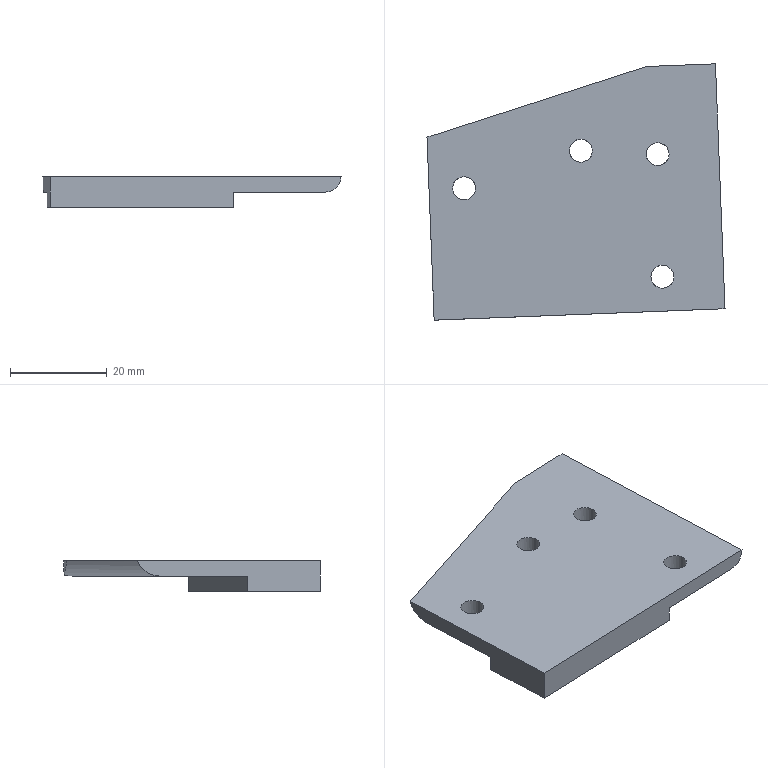Part | NX | features MG0301 nose pivot 24(right) 2 | 1 solid | 14 faces | box 61.764 x 53.123 x 6.35 mm | volume 10727 mm3 | plane 8 | cylinder 6 | commonest cylinder face diameters 4.763 x4 6.35 x1 9.525 x1
STEP:
#1=CARTESIAN_POINT('',(-3.173,-0.1243,6.35));
#2=VERTEX_POINT('',#1);
#3=CARTESIAN_POINT('',(-5.334,-0.209,3.34));
#4=VERTEX_POINT('',#3);
#5=CARTESIAN_POINT('',(-6.345,-0.2486,6.35));
#6=DIRECTION('',(0.03915,-0.9992,0.));
#7=DIRECTION('',(-0.9992,-0.03915,0.));
#8=AXIS2_PLACEMENT_3D('',#5,#6,#7);
#9=CIRCLE('',#8,3.175);
#10=EDGE_CURVE('',#2,#4,#9,.F.);
#11=ORIENTED_EDGE('',*,*,#10,.T.);
#12=CARTESIAN_POINT('',(-17.397,-0.6816,6.35));
#13=VERTEX_POINT('',#12);
#14=CARTESIAN_POINT('',(-0.7099,-0.02781,7.938));
#15=DIRECTION('',(0.03915,-0.9992,0.));
#16=DIRECTION('',(0.9992,0.03915,0.));
#17=AXIS2_PLACEMENT_3D('',#14,#15,#16);
#18=ELLIPSE('',#17,17.713,4.763);
#19=EDGE_CURVE('',#4,#13,#18,.F.);
#20=ORIENTED_EDGE('',*,*,#19,.T.);
#21=CARTESIAN_POINT('',(0.,0.,6.35));
#22=DIRECTION('',(-0.9992,-0.03915,0.));
#23=VECTOR('',#22,1000.);
#24=LINE('',#21,#23);
#25=EDGE_CURVE('',#2,#13,#24,.T.);
#26=ORIENTED_EDGE('',*,*,#25,.F.);
#27=EDGE_LOOP('',(#11,#20,#26));
#28=FACE_BOUND('',#27,.T.);
#29=CARTESIAN_POINT('',(0.,0.,6.35));
#30=DIRECTION('',(-0.03915,0.9992,0.));
#31=DIRECTION('',(-0.9992,-0.03915,0.));
#32=AXIS2_PLACEMENT_3D('',#29,#30,#31);
#33=PLANE('',#32);
#34=ADVANCED_FACE('',(#28),#33,.T.);
#35=CARTESIAN_POINT('',(-23.392,-51.755,0.));
#36=VERTEX_POINT('',#35);
#37=CARTESIAN_POINT('',(-23.392,-51.755,3.175));
#38=VERTEX_POINT('',#37);
#39=CARTESIAN_POINT('',(-23.392,-51.755,6.35));
#40=DIRECTION('',(0.,0.,1.));
#41=VECTOR('',#40,1000.);
#42=LINE('',#39,#41);
#43=EDGE_CURVE('',#36,#38,#42,.T.);
#44=ORIENTED_EDGE('',*,*,#43,.T.);
#45=CARTESIAN_POINT('',(-4.357,-51.01,3.175));
#46=VERTEX_POINT('',#45);
#47=CARTESIAN_POINT('',(-61.463,-53.247,3.175));
#48=DIRECTION('',(0.9992,0.03915,0.));
#49=VECTOR('',#48,1000.);
#50=LINE('',#47,#49);
#51=EDGE_CURVE('',#38,#46,#50,.T.);
#52=ORIENTED_EDGE('',*,*,#51,.T.);
#53=CARTESIAN_POINT('',(-1.184,-50.885,6.35));
#54=VERTEX_POINT('',#53);
#55=CARTESIAN_POINT('',(-4.357,-51.01,6.35));
#56=DIRECTION('',(-0.03915,0.9992,0.));
#57=DIRECTION('',(0.9992,0.03915,0.));
#58=AXIS2_PLACEMENT_3D('',#55,#56,#57);
#59=CIRCLE('',#58,3.175);
#60=EDGE_CURVE('',#46,#54,#59,.F.);
#61=ORIENTED_EDGE('',*,*,#60,.T.);
#62=CARTESIAN_POINT('',(-61.463,-53.247,6.35));
#63=VERTEX_POINT('',#62);
#64=CARTESIAN_POINT('',(-61.463,-53.247,6.35));
#65=DIRECTION('',(0.9992,0.03915,0.));
#66=VECTOR('',#65,1000.);
#67=LINE('',#64,#66);
#68=EDGE_CURVE('',#63,#54,#67,.T.);
#69=ORIENTED_EDGE('',*,*,#68,.F.);
#70=CARTESIAN_POINT('',(-61.463,-53.247,0.));
#71=VERTEX_POINT('',#70);
#72=CARTESIAN_POINT('',(-61.463,-53.247,6.35));
#73=DIRECTION('',(0.,0.,-1.));
#74=VECTOR('',#73,1000.);
#75=LINE('',#72,#74);
#76=EDGE_CURVE('',#63,#71,#75,.T.);
#77=ORIENTED_EDGE('',*,*,#76,.T.);
#78=CARTESIAN_POINT('',(-61.463,-53.247,0.));
#79=DIRECTION('',(0.9992,0.03915,0.));
#80=VECTOR('',#79,1000.);
#81=LINE('',#78,#80);
#82=EDGE_CURVE('',#71,#36,#81,.T.);
#83=ORIENTED_EDGE('',*,*,#82,.T.);
#84=EDGE_LOOP('',(#44,#52,#61,#69,#77,#83));
#85=FACE_BOUND('',#84,.T.);
#86=CARTESIAN_POINT('',(-61.463,-53.247,6.35));
#87=DIRECTION('',(0.03915,-0.9992,0.));
#88=DIRECTION('',(0.9992,0.03915,0.));
#89=AXIS2_PLACEMENT_3D('',#86,#87,#88);
#90=PLANE('',#89);
#91=ADVANCED_FACE('',(#85),#90,.T.);
#92=CARTESIAN_POINT('',(-15.149,-16.459,3.175));
#93=VERTEX_POINT('',#92);
#94=CARTESIAN_POINT('',(-15.149,-18.84,3.175));
#95=DIRECTION('',(0.,0.,-1.));
#96=DIRECTION('',(0.,1.,0.));
#97=AXIS2_PLACEMENT_3D('',#94,#95,#96);
#98=CIRCLE('',#97,2.381);
#99=EDGE_CURVE('',#93,#93,#98,.T.);
#100=ORIENTED_EDGE('',*,*,#99,.F.);
#101=EDGE_LOOP('',(#100));
#102=FACE_BOUND('',#101,.T.);
#103=CARTESIAN_POINT('',(-31.064,-15.754,3.175));
#104=VERTEX_POINT('',#103);
#105=CARTESIAN_POINT('',(-31.064,-18.135,3.175));
#106=DIRECTION('',(0.,0.,-1.));
#107=DIRECTION('',(0.,1.,0.));
#108=AXIS2_PLACEMENT_3D('',#105,#106,#107);
#109=CIRCLE('',#108,2.381);
#110=EDGE_CURVE('',#104,#104,#109,.T.);
#111=ORIENTED_EDGE('',*,*,#110,.F.);
#112=EDGE_LOOP('',(#111));
#113=FACE_BOUND('',#112,.T.);
#114=CARTESIAN_POINT('',(-55.242,-23.536,3.175));
#115=VERTEX_POINT('',#114);
#116=CARTESIAN_POINT('',(-55.242,-25.917,3.175));
#117=DIRECTION('',(0.,0.,-1.));
#118=DIRECTION('',(0.,1.,0.));
#119=AXIS2_PLACEMENT_3D('',#116,#117,#118);
#120=CIRCLE('',#119,2.381);
#121=EDGE_CURVE('',#115,#115,#120,.T.);
#122=ORIENTED_EDGE('',*,*,#121,.F.);
#123=EDGE_LOOP('',(#122));
#124=FACE_BOUND('',#123,.T.);
#125=CARTESIAN_POINT('',(-14.154,-41.859,3.175));
#126=VERTEX_POINT('',#125);
#127=CARTESIAN_POINT('',(-14.154,-44.24,3.175));
#128=DIRECTION('',(0.,0.,-1.));
#129=DIRECTION('',(0.,1.,0.));
#130=AXIS2_PLACEMENT_3D('',#127,#128,#129);
#131=CIRCLE('',#130,2.381);
#132=EDGE_CURVE('',#126,#126,#131,.T.);
#133=ORIENTED_EDGE('',*,*,#132,.F.);
#134=EDGE_LOOP('',(#133));
#135=FACE_BOUND('',#134,.T.);
#136=CARTESIAN_POINT('',(-62.055,-38.116,3.175));
#137=VERTEX_POINT('',#136);
#138=CARTESIAN_POINT('',(-24.401,-25.997,3.175));
#139=VERTEX_POINT('',#138);
#140=CARTESIAN_POINT('',(-468.479,-168.921,3.175));
#141=DIRECTION('',(0.9519,0.3064,0.));
#142=VECTOR('',#141,1000.);
#143=LINE('',#140,#142);
#144=EDGE_CURVE('',#137,#139,#143,.T.);
#145=ORIENTED_EDGE('',*,*,#144,.F.);
#146=CARTESIAN_POINT('',(-62.765,-20.,3.175));
#147=VERTEX_POINT('',#146);
#148=CARTESIAN_POINT('',(-62.959,-15.059,3.175));
#149=DIRECTION('',(0.03915,-0.9992,0.));
#150=VECTOR('',#149,1000.);
#151=LINE('',#148,#150);
#152=EDGE_CURVE('',#147,#137,#151,.T.);
#153=ORIENTED_EDGE('',*,*,#152,.F.);
#154=CARTESIAN_POINT('',(-6.284,-1.822,3.175));
#155=VERTEX_POINT('',#154);
#156=CARTESIAN_POINT('',(-473.829,-152.298,3.175));
#157=DIRECTION('',(0.9519,0.3064,0.));
#158=VECTOR('',#157,1000.);
#159=LINE('',#156,#158);
#160=EDGE_CURVE('',#147,#155,#159,.T.);
#161=ORIENTED_EDGE('',*,*,#160,.T.);
#162=CARTESIAN_POINT('',(13.897,-516.93,3.175));
#163=DIRECTION('',(-0.03915,0.9992,0.));
#164=VECTOR('',#163,1000.);
#165=LINE('',#162,#164);
#166=EDGE_CURVE('',#46,#155,#165,.T.);
#167=ORIENTED_EDGE('',*,*,#166,.F.);
#168=ORIENTED_EDGE('',*,*,#51,.F.);
#169=CARTESIAN_POINT('',(-5.139,-517.676,3.175));
#170=DIRECTION('',(-0.03915,0.9992,0.));
#171=VECTOR('',#170,1000.);
#172=LINE('',#169,#171);
#173=EDGE_CURVE('',#38,#139,#172,.T.);
#174=ORIENTED_EDGE('',*,*,#173,.T.);
#175=EDGE_LOOP('',(#145,#153,#161,#167,#168,#174));
#176=FACE_BOUND('',#175,.T.);
#177=CARTESIAN_POINT('',(-468.479,-168.921,3.175));
#178=DIRECTION('',(0.,0.,1.));
#179=DIRECTION('',(0.,1.,0.));
#180=AXIS2_PLACEMENT_3D('',#177,#178,#179);
#181=PLANE('',#180);
#182=ADVANCED_FACE('',(#102,#113,#124,#135,#176),#181,.F.);
#183=CARTESIAN_POINT('',(-62.055,-38.116,0.));
#184=VERTEX_POINT('',#183);
#185=CARTESIAN_POINT('',(-24.401,-25.997,0.));
#186=VERTEX_POINT('',#185);
#187=CARTESIAN_POINT('',(-52.929,-35.179,0.));
#188=DIRECTION('',(0.9519,0.3064,0.));
#189=VECTOR('',#188,1000.);
#190=LINE('',#187,#189);
#191=EDGE_CURVE('',#184,#186,#190,.T.);
#192=ORIENTED_EDGE('',*,*,#191,.F.);
#193=CARTESIAN_POINT('',(-62.055,-38.116,6.35));
#194=DIRECTION('',(0.,0.,-1.));
#195=VECTOR('',#194,1000.);
#196=LINE('',#193,#195);
#197=EDGE_CURVE('',#137,#184,#196,.T.);
#198=ORIENTED_EDGE('',*,*,#197,.F.);
#199=ORIENTED_EDGE('',*,*,#144,.T.);
#200=CARTESIAN_POINT('',(-24.401,-25.997,0.));
#201=DIRECTION('',(0.,0.,1.));
#202=VECTOR('',#201,1000.);
#203=LINE('',#200,#202);
#204=EDGE_CURVE('',#186,#139,#203,.T.);
#205=ORIENTED_EDGE('',*,*,#204,.F.);
#206=EDGE_LOOP('',(#192,#198,#199,#205));
#207=FACE_BOUND('',#206,.T.);
#208=CARTESIAN_POINT('',(-468.479,-168.921,0.));
#209=DIRECTION('',(0.3064,-0.9519,0.));
#210=DIRECTION('',(0.9519,0.3064,0.));
#211=AXIS2_PLACEMENT_3D('',#208,#209,#210);
#212=PLANE('',#211);
#213=ADVANCED_FACE('',(#207),#212,.F.);
#214=CARTESIAN_POINT('',(-62.948,-15.342,6.35));
#215=VERTEX_POINT('',#214);
#216=CARTESIAN_POINT('',(-62.765,-20.,7.938));
#217=DIRECTION('',(0.9992,0.03915,0.));
#218=DIRECTION('',(-0.03915,0.9992,0.));
#219=AXIS2_PLACEMENT_3D('',#216,#217,#218);
#220=ELLIPSE('',#219,4.945,4.763);
#221=EDGE_CURVE('',#215,#147,#220,.F.);
#222=ORIENTED_EDGE('',*,*,#221,.T.);
#223=ORIENTED_EDGE('',*,*,#152,.T.);
#224=ORIENTED_EDGE('',*,*,#197,.T.);
#225=CARTESIAN_POINT('',(-62.959,-15.059,0.));
#226=DIRECTION('',(0.03915,-0.9992,0.));
#227=VECTOR('',#226,1000.);
#228=LINE('',#225,#227);
#229=EDGE_CURVE('',#184,#71,#228,.T.);
#230=ORIENTED_EDGE('',*,*,#229,.T.);
#231=ORIENTED_EDGE('',*,*,#76,.F.);
#232=CARTESIAN_POINT('',(-62.959,-15.059,6.35));
#233=DIRECTION('',(0.03915,-0.9992,0.));
#234=VECTOR('',#233,1000.);
#235=LINE('',#232,#234);
#236=EDGE_CURVE('',#215,#63,#235,.T.);
#237=ORIENTED_EDGE('',*,*,#236,.F.);
#238=EDGE_LOOP('',(#222,#223,#224,#230,#231,#237));
#239=FACE_BOUND('',#238,.T.);
#240=CARTESIAN_POINT('',(-62.959,-15.059,6.35));
#241=DIRECTION('',(-0.9992,-0.03915,0.));
#242=DIRECTION('',(0.03915,-0.9992,0.));
#243=AXIS2_PLACEMENT_3D('',#240,#241,#242);
#244=PLANE('',#243);
#245=ADVANCED_FACE('',(#239),#244,.T.);
#246=CARTESIAN_POINT('',(-28.683,-18.135,6.35));
#247=VERTEX_POINT('',#246);
#248=CARTESIAN_POINT('',(-31.064,-18.135,6.35));
#249=DIRECTION('',(0.,0.,1.));
#250=DIRECTION('',(1.,0.,0.));
#251=AXIS2_PLACEMENT_3D('',#248,#249,#250);
#252=CIRCLE('',#251,2.381);
#253=EDGE_CURVE('',#247,#247,#252,.T.);
#254=ORIENTED_EDGE('',*,*,#253,.F.);
#255=EDGE_LOOP('',(#254));
#256=FACE_BOUND('',#255,.T.);
#257=CARTESIAN_POINT('',(-52.861,-25.917,6.35));
#258=VERTEX_POINT('',#257);
#259=CARTESIAN_POINT('',(-55.242,-25.917,6.35));
#260=DIRECTION('',(0.,0.,1.));
#261=DIRECTION('',(1.,0.,0.));
#262=AXIS2_PLACEMENT_3D('',#259,#260,#261);
#263=CIRCLE('',#262,2.381);
#264=EDGE_CURVE('',#258,#258,#263,.T.);
#265=ORIENTED_EDGE('',*,*,#264,.F.);
#266=EDGE_LOOP('',(#265));
#267=FACE_BOUND('',#266,.T.);
#268=CARTESIAN_POINT('',(-11.773,-44.24,6.35));
#269=VERTEX_POINT('',#268);
#270=CARTESIAN_POINT('',(-14.154,-44.24,6.35));
#271=DIRECTION('',(0.,0.,1.));
#272=DIRECTION('',(1.,0.,0.));
#273=AXIS2_PLACEMENT_3D('',#270,#271,#272);
#274=CIRCLE('',#273,2.381);
#275=EDGE_CURVE('',#269,#269,#274,.T.);
#276=ORIENTED_EDGE('',*,*,#275,.F.);
#277=EDGE_LOOP('',(#276));
#278=FACE_BOUND('',#277,.T.);
#279=ORIENTED_EDGE('',*,*,#25,.T.);
#280=CARTESIAN_POINT('',(-475.205,-148.024,6.35));
#281=DIRECTION('',(0.9519,0.3064,0.));
#282=VECTOR('',#281,1000.);
#283=LINE('',#280,#282);
#284=EDGE_CURVE('',#215,#13,#283,.T.);
#285=ORIENTED_EDGE('',*,*,#284,.F.);
#286=ORIENTED_EDGE('',*,*,#236,.T.);
#287=ORIENTED_EDGE('',*,*,#68,.T.);
#288=CARTESIAN_POINT('',(17.069,-516.806,6.35));
#289=DIRECTION('',(-0.03915,0.9992,0.));
#290=VECTOR('',#289,1000.);
#291=LINE('',#288,#290);
#292=EDGE_CURVE('',#54,#2,#291,.T.);
#293=ORIENTED_EDGE('',*,*,#292,.T.);
#294=EDGE_LOOP('',(#279,#285,#286,#287,#293));
#295=FACE_BOUND('',#294,.T.);
#296=CARTESIAN_POINT('',(-12.768,-18.84,6.35));
#297=VERTEX_POINT('',#296);
#298=CARTESIAN_POINT('',(-15.149,-18.84,6.35));
#299=DIRECTION('',(0.,0.,1.));
#300=DIRECTION('',(1.,0.,0.));
#301=AXIS2_PLACEMENT_3D('',#298,#299,#300);
#302=CIRCLE('',#301,2.381);
#303=EDGE_CURVE('',#297,#297,#302,.T.);
#304=ORIENTED_EDGE('',*,*,#303,.F.);
#305=EDGE_LOOP('',(#304));
#306=FACE_BOUND('',#305,.T.);
#307=CARTESIAN_POINT('',(-63.451,-2.486,6.35));
#308=DIRECTION('',(0.,0.,-1.));
#309=DIRECTION('',(1.,0.,0.));
#310=AXIS2_PLACEMENT_3D('',#307,#308,#309);
#311=PLANE('',#310);
#312=ADVANCED_FACE('',(#256,#267,#278,#295,#306),#311,.F.);
#313=CARTESIAN_POINT('',(-5.139,-517.676,0.));
#314=DIRECTION('',(-0.03915,0.9992,0.));
#315=VECTOR('',#314,1000.);
#316=LINE('',#313,#315);
#317=EDGE_CURVE('',#36,#186,#316,.T.);
#318=ORIENTED_EDGE('',*,*,#317,.F.);
#319=ORIENTED_EDGE('',*,*,#82,.F.);
#320=ORIENTED_EDGE('',*,*,#229,.F.);
#321=ORIENTED_EDGE('',*,*,#191,.T.);
#322=EDGE_LOOP('',(#318,#319,#320,#321));
#323=FACE_BOUND('',#322,.T.);
#324=CARTESIAN_POINT('',(-63.451,-2.486,0.));
#325=DIRECTION('',(0.,0.,-1.));
#326=DIRECTION('',(1.,0.,0.));
#327=AXIS2_PLACEMENT_3D('',#324,#325,#326);
#328=PLANE('',#327);
#329=ADVANCED_FACE('',(#323),#328,.T.);
#330=ORIENTED_EDGE('',*,*,#160,.F.);
#331=ORIENTED_EDGE('',*,*,#221,.F.);
#332=ORIENTED_EDGE('',*,*,#284,.T.);
#333=ORIENTED_EDGE('',*,*,#19,.F.);
#334=CARTESIAN_POINT('',(-5.334,-0.209,3.34));
#335=CARTESIAN_POINT('',(-5.645,-0.741,3.229));
#336=CARTESIAN_POINT('',(-5.964,-1.281,3.175));
#337=CARTESIAN_POINT('',(-6.284,-1.822,3.175));
#338=B_SPLINE_CURVE_WITH_KNOTS('',3,(#334,#335,#336,#337),.UNSPECIFIED.,.F.,.F.,(4,4),(0.005677,0.007559),.UNSPECIFIED.);
#339=EDGE_CURVE('',#155,#4,#338,.F.);
#340=ORIENTED_EDGE('',*,*,#339,.F.);
#341=EDGE_LOOP('',(#330,#331,#332,#333,#340));
#342=FACE_BOUND('',#341,.T.);
#343=CARTESIAN_POINT('',(-473.829,-152.298,7.938));
#344=DIRECTION('',(0.9519,0.3064,0.));
#345=DIRECTION('',(-0.3064,0.9519,0.));
#346=AXIS2_PLACEMENT_3D('',#343,#344,#345);
#347=CYLINDRICAL_SURFACE('',#346,4.763);
#348=ADVANCED_FACE('',(#342),#347,.T.);
#349=ORIENTED_EDGE('',*,*,#43,.F.);
#350=ORIENTED_EDGE('',*,*,#317,.T.);
#351=ORIENTED_EDGE('',*,*,#204,.T.);
#352=ORIENTED_EDGE('',*,*,#173,.F.);
#353=EDGE_LOOP('',(#349,#350,#351,#352));
#354=FACE_BOUND('',#353,.T.);
#355=CARTESIAN_POINT('',(-5.139,-517.676,0.));
#356=DIRECTION('',(-0.9992,-0.03915,0.));
#357=DIRECTION('',(0.03915,-0.9992,0.));
#358=AXIS2_PLACEMENT_3D('',#355,#356,#357);
#359=PLANE('',#358);
#360=ADVANCED_FACE('',(#354),#359,.F.);
#361=ORIENTED_EDGE('',*,*,#60,.F.);
#362=ORIENTED_EDGE('',*,*,#166,.T.);
#363=ORIENTED_EDGE('',*,*,#339,.T.);
#364=ORIENTED_EDGE('',*,*,#10,.F.);
#365=ORIENTED_EDGE('',*,*,#292,.F.);
#366=EDGE_LOOP('',(#361,#362,#363,#364,#365));
#367=FACE_BOUND('',#366,.T.);
#368=CARTESIAN_POINT('',(13.897,-516.93,6.35));
#369=DIRECTION('',(-0.03915,0.9992,0.));
#370=DIRECTION('',(-0.9992,-0.03915,0.));
#371=AXIS2_PLACEMENT_3D('',#368,#369,#370);
#372=CYLINDRICAL_SURFACE('',#371,3.175);
#373=ADVANCED_FACE('',(#367),#372,.T.);
#374=ORIENTED_EDGE('',*,*,#303,.T.);
#375=EDGE_LOOP('',(#374));
#376=FACE_BOUND('',#375,.T.);
#377=ORIENTED_EDGE('',*,*,#99,.T.);
#378=EDGE_LOOP('',(#377));
#379=FACE_BOUND('',#378,.T.);
#380=CARTESIAN_POINT('',(-15.149,-18.84,63.5));
#381=DIRECTION('',(0.,0.,-1.));
#382=DIRECTION('',(1.,0.,0.));
#383=AXIS2_PLACEMENT_3D('',#380,#381,#382);
#384=CYLINDRICAL_SURFACE('',#383,2.381);
#385=ADVANCED_FACE('',(#376,#379),#384,.F.);
#386=ORIENTED_EDGE('',*,*,#275,.T.);
#387=EDGE_LOOP('',(#386));
#388=FACE_BOUND('',#387,.T.);
#389=ORIENTED_EDGE('',*,*,#132,.T.);
#390=EDGE_LOOP('',(#389));
#391=FACE_BOUND('',#390,.T.);
#392=CARTESIAN_POINT('',(-14.154,-44.24,63.5));
#393=DIRECTION('',(0.,0.,-1.));
#394=DIRECTION('',(1.,0.,0.));
#395=AXIS2_PLACEMENT_3D('',#392,#393,#394);
#396=CYLINDRICAL_SURFACE('',#395,2.381);
#397=ADVANCED_FACE('',(#388,#391),#396,.F.);
#398=ORIENTED_EDGE('',*,*,#264,.T.);
#399=EDGE_LOOP('',(#398));
#400=FACE_BOUND('',#399,.T.);
#401=ORIENTED_EDGE('',*,*,#121,.T.);
#402=EDGE_LOOP('',(#401));
#403=FACE_BOUND('',#402,.T.);
#404=CARTESIAN_POINT('',(-55.242,-25.917,63.5));
#405=DIRECTION('',(0.,0.,-1.));
#406=DIRECTION('',(1.,0.,0.));
#407=AXIS2_PLACEMENT_3D('',#404,#405,#406);
#408=CYLINDRICAL_SURFACE('',#407,2.381);
#409=ADVANCED_FACE('',(#400,#403),#408,.F.);
#410=ORIENTED_EDGE('',*,*,#253,.T.);
#411=EDGE_LOOP('',(#410));
#412=FACE_BOUND('',#411,.T.);
#413=ORIENTED_EDGE('',*,*,#110,.T.);
#414=EDGE_LOOP('',(#413));
#415=FACE_BOUND('',#414,.T.);
#416=CARTESIAN_POINT('',(-31.064,-18.135,63.5));
#417=DIRECTION('',(0.,0.,-1.));
#418=DIRECTION('',(1.,0.,0.));
#419=AXIS2_PLACEMENT_3D('',#416,#417,#418);
#420=CYLINDRICAL_SURFACE('',#419,2.381);
#421=ADVANCED_FACE('',(#412,#415),#420,.F.);
#422=CLOSED_SHELL('',(#34,#91,#182,#213,#245,#312,#329,#348,#360,#373,#385,#397,#409,#421));
#423=MANIFOLD_SOLID_BREP('',#422);
#424=(LENGTH_UNIT()NAMED_UNIT(*)SI_UNIT(.MILLI.,.METRE.));
#425=UNCERTAINTY_MEASURE_WITH_UNIT(LENGTH_MEASURE(0.0508),#424,'','');
#426=(NAMED_UNIT(*)PLANE_ANGLE_UNIT()SI_UNIT($,.RADIAN.));
#427=(NAMED_UNIT(*)SI_UNIT($,.STERADIAN.)SOLID_ANGLE_UNIT());
#428=(GEOMETRIC_REPRESENTATION_CONTEXT(3)GLOBAL_UNCERTAINTY_ASSIGNED_CONTEXT((#425))GLOBAL_UNIT_ASSIGNED_CONTEXT((#424,#426,#427))REPRESENTATION_CONTEXT('',''));
#429=ADVANCED_BREP_SHAPE_REPRESENTATION('',(#423),#428);